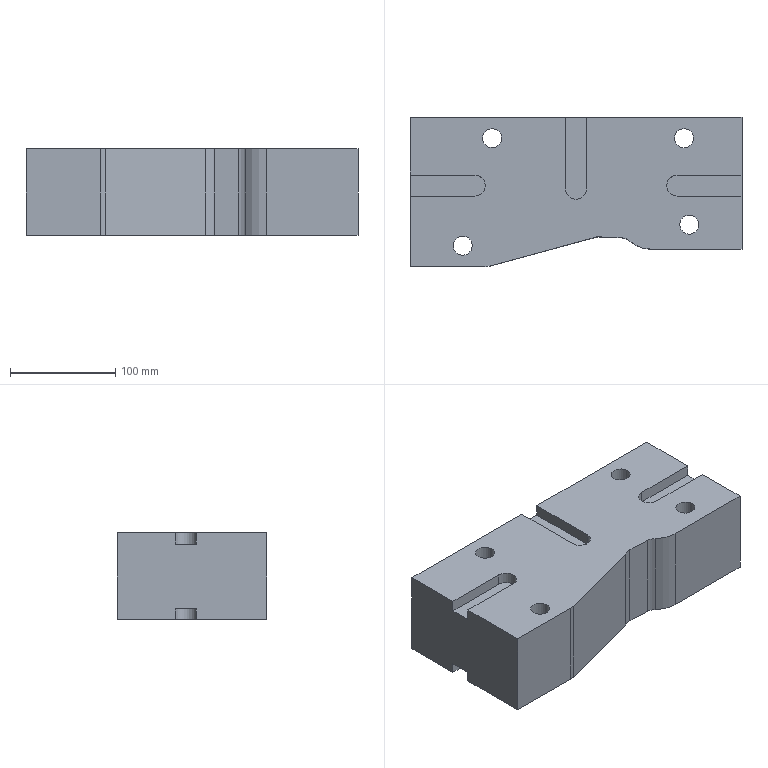Part | STEP file | lll_id2490_x_t | 1 solid | 69 faces | box 315 x 142 x 82.5 mm | volume 3094581 mm3 | plane 31 | cylinder 25 | cone 10 | spline 3 | commonest cylinder face diameters 6.8 x6 20 x6 14.506 x4 18.009 x4 26.007 x4 30 x1